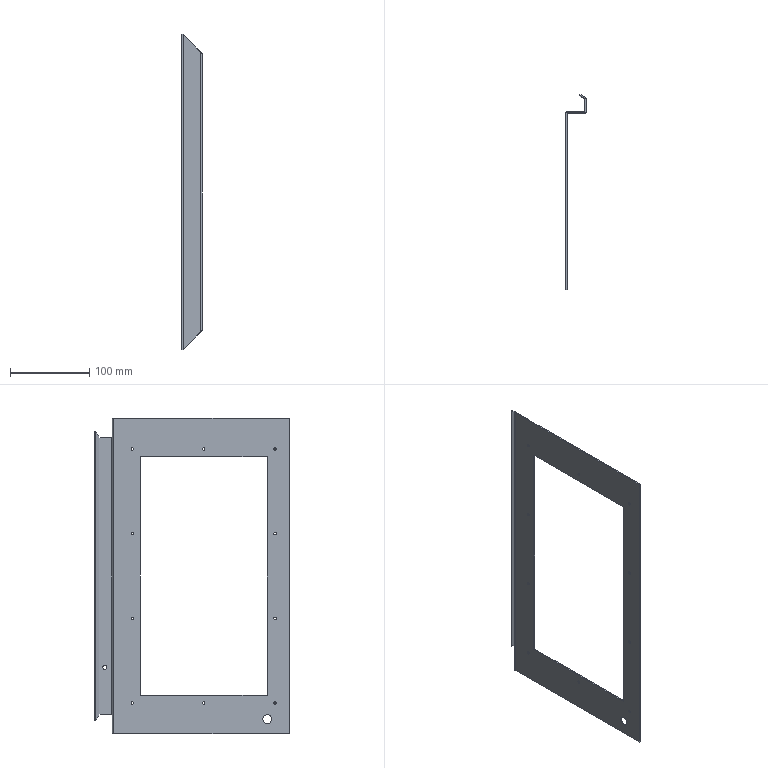Part | SolidWorks | features Cut 4, FlatPattern 1, SMBaseFlange 1, SheetMetal 1 | 1 solid | 60 faces | box 25.5 x 245.5 x 397 mm | volume 87187 mm3 | cylinder 30 | plane 26 | spline 4 | commonest cylinder face diameters 3.2 x20 0.6 x3 3.6 x3 5.2 x2 11 x2